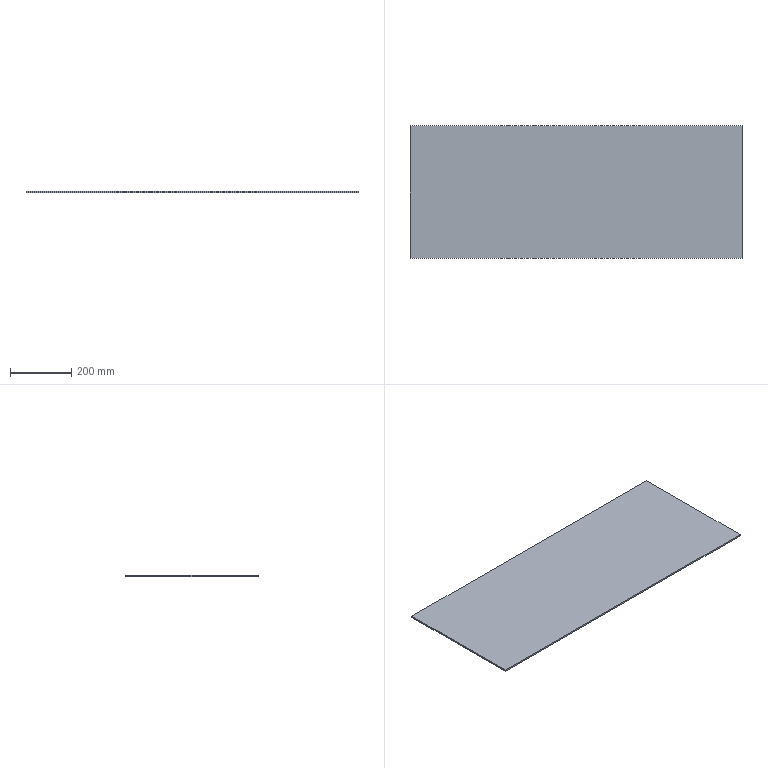Part | STEP file | Vibration-damping sponge | 1 solid | 6 faces | box 1080 x 430 x 5 mm | volume 2322000 mm3 | plane 6
STEP:
#1=CARTESIAN_POINT('',(0.,0.,0.));
#2=DIRECTION('',(0.,0.,1.));
#3=DIRECTION('',(1.,0.,0.));
#4=AXIS2_PLACEMENT_3D('',#1,#2,#3);
#5=CARTESIAN_POINT('',(-540.,215.,0.));
#6=VERTEX_POINT('',#5);
#7=CARTESIAN_POINT('',(-540.,-215.,0.));
#8=VERTEX_POINT('',#7);
#9=CARTESIAN_POINT('',(-540.,215.,0.));
#10=DIRECTION('',(0.,-1.,0.));
#11=VECTOR('',#10,1.);
#12=LINE('',#9,#11);
#13=CARTESIAN_POINT('',(-540.,215.,5.));
#14=DIRECTION('',(1.,0.,0.));
#15=DIRECTION('',(0.,0.,-1.));
#16=AXIS2_PLACEMENT_3D('',#13,#14,#15);
#17=PLANE('',#16);
#18=CARTESIAN_POINT('',(5.,0.));
#19=DIRECTION('',(0.,-1.));
#20=VECTOR('',#19,1.);
#21=LINE('',#18,#20);
#22=(GEOMETRIC_REPRESENTATION_CONTEXT(2)PARAMETRIC_REPRESENTATION_CONTEXT()REPRESENTATION_CONTEXT('',''));
#23=DEFINITIONAL_REPRESENTATION('',(#21),#22);
#24=PCURVE('',#17,#23);
#25=CARTESIAN_POINT('',(-540.,-215.,0.));
#26=DIRECTION('',(0.,0.,1.));
#27=DIRECTION('',(1.,0.,0.));
#28=AXIS2_PLACEMENT_3D('',#25,#26,#27);
#29=PLANE('',#28);
#30=CARTESIAN_POINT('',(0.,430.));
#31=DIRECTION('',(0.,-1.));
#32=VECTOR('',#31,1.);
#33=LINE('',#30,#32);
#34=(GEOMETRIC_REPRESENTATION_CONTEXT(2)PARAMETRIC_REPRESENTATION_CONTEXT()REPRESENTATION_CONTEXT('',''));
#35=DEFINITIONAL_REPRESENTATION('',(#33),#34);
#36=PCURVE('',#29,#35);
#37=SURFACE_CURVE('',#12,(#24,#36),.PCURVE_S1.);
#38=EDGE_CURVE('',#6,#8,#37,.T.);
#39=ORIENTED_EDGE('',*,*,#38,.T.);
#40=CARTESIAN_POINT('',(-540.,-215.,5.));
#41=VERTEX_POINT('',#40);
#42=CARTESIAN_POINT('',(-540.,-215.,5.));
#43=DIRECTION('',(0.,0.,-1.));
#44=VECTOR('',#43,1.);
#45=LINE('',#42,#44);
#46=CARTESIAN_POINT('',(0.,-430.));
#47=DIRECTION('',(1.,0.));
#48=VECTOR('',#47,1.);
#49=LINE('',#46,#48);
#50=(GEOMETRIC_REPRESENTATION_CONTEXT(2)PARAMETRIC_REPRESENTATION_CONTEXT()REPRESENTATION_CONTEXT('',''));
#51=DEFINITIONAL_REPRESENTATION('',(#49),#50);
#52=PCURVE('',#17,#51);
#53=CARTESIAN_POINT('',(-540.,-215.,5.));
#54=DIRECTION('',(0.,1.,0.));
#55=DIRECTION('',(0.,0.,1.));
#56=AXIS2_PLACEMENT_3D('',#53,#54,#55);
#57=PLANE('',#56);
#58=CARTESIAN_POINT('',(0.,0.));
#59=DIRECTION('',(-1.,0.));
#60=VECTOR('',#59,1.);
#61=LINE('',#58,#60);
#62=(GEOMETRIC_REPRESENTATION_CONTEXT(2)PARAMETRIC_REPRESENTATION_CONTEXT()REPRESENTATION_CONTEXT('',''));
#63=DEFINITIONAL_REPRESENTATION('',(#61),#62);
#64=PCURVE('',#57,#63);
#65=SURFACE_CURVE('',#45,(#52,#64),.PCURVE_S1.);
#66=EDGE_CURVE('',#41,#8,#65,.T.);
#67=ORIENTED_EDGE('',*,*,#66,.F.);
#68=CARTESIAN_POINT('',(-540.,215.,5.));
#69=VERTEX_POINT('',#68);
#70=CARTESIAN_POINT('',(-540.,215.,5.));
#71=DIRECTION('',(0.,-1.,0.));
#72=VECTOR('',#71,1.);
#73=LINE('',#70,#72);
#74=CARTESIAN_POINT('',(0.,0.));
#75=DIRECTION('',(0.,-1.));
#76=VECTOR('',#75,1.);
#77=LINE('',#74,#76);
#78=(GEOMETRIC_REPRESENTATION_CONTEXT(2)PARAMETRIC_REPRESENTATION_CONTEXT()REPRESENTATION_CONTEXT('',''));
#79=DEFINITIONAL_REPRESENTATION('',(#77),#78);
#80=PCURVE('',#17,#79);
#81=CARTESIAN_POINT('',(-540.,-215.,5.));
#82=DIRECTION('',(0.,0.,1.));
#83=DIRECTION('',(1.,0.,0.));
#84=AXIS2_PLACEMENT_3D('',#81,#82,#83);
#85=PLANE('',#84);
#86=CARTESIAN_POINT('',(0.,430.));
#87=DIRECTION('',(0.,-1.));
#88=VECTOR('',#87,1.);
#89=LINE('',#86,#88);
#90=(GEOMETRIC_REPRESENTATION_CONTEXT(2)PARAMETRIC_REPRESENTATION_CONTEXT()REPRESENTATION_CONTEXT('',''));
#91=DEFINITIONAL_REPRESENTATION('',(#89),#90);
#92=PCURVE('',#85,#91);
#93=SURFACE_CURVE('',#73,(#80,#92),.PCURVE_S1.);
#94=EDGE_CURVE('',#69,#41,#93,.T.);
#95=ORIENTED_EDGE('',*,*,#94,.F.);
#96=CARTESIAN_POINT('',(-540.,215.,5.));
#97=DIRECTION('',(0.,0.,-1.));
#98=VECTOR('',#97,1.);
#99=LINE('',#96,#98);
#100=CARTESIAN_POINT('',(0.,0.));
#101=DIRECTION('',(1.,0.));
#102=VECTOR('',#101,1.);
#103=LINE('',#100,#102);
#104=(GEOMETRIC_REPRESENTATION_CONTEXT(2)PARAMETRIC_REPRESENTATION_CONTEXT()REPRESENTATION_CONTEXT('',''));
#105=DEFINITIONAL_REPRESENTATION('',(#103),#104);
#106=PCURVE('',#17,#105);
#107=CARTESIAN_POINT('',(-540.,215.,5.));
#108=DIRECTION('',(0.,-1.,0.));
#109=DIRECTION('',(0.,0.,-1.));
#110=AXIS2_PLACEMENT_3D('',#107,#108,#109);
#111=PLANE('',#110);
#112=CARTESIAN_POINT('',(0.,0.));
#113=DIRECTION('',(1.,0.));
#114=VECTOR('',#113,1.);
#115=LINE('',#112,#114);
#116=(GEOMETRIC_REPRESENTATION_CONTEXT(2)PARAMETRIC_REPRESENTATION_CONTEXT()REPRESENTATION_CONTEXT('',''));
#117=DEFINITIONAL_REPRESENTATION('',(#115),#116);
#118=PCURVE('',#111,#117);
#119=SURFACE_CURVE('',#99,(#106,#118),.PCURVE_S1.);
#120=EDGE_CURVE('',#69,#6,#119,.T.);
#121=ORIENTED_EDGE('',*,*,#120,.T.);
#122=EDGE_LOOP('',(#39,#67,#95,#121));
#123=FACE_BOUND('',#122,.T.);
#124=ADVANCED_FACE('',(#123),#17,.F.);
#125=CARTESIAN_POINT('',(540.,-215.,0.));
#126=VERTEX_POINT('',#125);
#127=CARTESIAN_POINT('',(-540.,-215.,0.));
#128=DIRECTION('',(1.,0.,0.));
#129=VECTOR('',#128,1.);
#130=LINE('',#127,#129);
#131=CARTESIAN_POINT('',(-5.,0.));
#132=DIRECTION('',(0.,1.));
#133=VECTOR('',#132,1.);
#134=LINE('',#131,#133);
#135=(GEOMETRIC_REPRESENTATION_CONTEXT(2)PARAMETRIC_REPRESENTATION_CONTEXT()REPRESENTATION_CONTEXT('',''));
#136=DEFINITIONAL_REPRESENTATION('',(#134),#135);
#137=PCURVE('',#57,#136);
#138=CARTESIAN_POINT('',(0.,0.));
#139=DIRECTION('',(1.,0.));
#140=VECTOR('',#139,1.);
#141=LINE('',#138,#140);
#142=(GEOMETRIC_REPRESENTATION_CONTEXT(2)PARAMETRIC_REPRESENTATION_CONTEXT()REPRESENTATION_CONTEXT('',''));
#143=DEFINITIONAL_REPRESENTATION('',(#141),#142);
#144=PCURVE('',#29,#143);
#145=SURFACE_CURVE('',#130,(#137,#144),.PCURVE_S1.);
#146=EDGE_CURVE('',#8,#126,#145,.T.);
#147=ORIENTED_EDGE('',*,*,#146,.T.);
#148=CARTESIAN_POINT('',(540.,-215.,5.));
#149=VERTEX_POINT('',#148);
#150=CARTESIAN_POINT('',(540.,-215.,5.));
#151=DIRECTION('',(0.,0.,-1.));
#152=VECTOR('',#151,1.);
#153=LINE('',#150,#152);
#154=CARTESIAN_POINT('',(0.,1080.));
#155=DIRECTION('',(-1.,0.));
#156=VECTOR('',#155,1.);
#157=LINE('',#154,#156);
#158=(GEOMETRIC_REPRESENTATION_CONTEXT(2)PARAMETRIC_REPRESENTATION_CONTEXT()REPRESENTATION_CONTEXT('',''));
#159=DEFINITIONAL_REPRESENTATION('',(#157),#158);
#160=PCURVE('',#57,#159);
#161=CARTESIAN_POINT('',(540.,215.,5.));
#162=DIRECTION('',(-1.,0.,0.));
#163=DIRECTION('',(0.,0.,1.));
#164=AXIS2_PLACEMENT_3D('',#161,#162,#163);
#165=PLANE('',#164);
#166=CARTESIAN_POINT('',(0.,-430.));
#167=DIRECTION('',(-1.,0.));
#168=VECTOR('',#167,1.);
#169=LINE('',#166,#168);
#170=(GEOMETRIC_REPRESENTATION_CONTEXT(2)PARAMETRIC_REPRESENTATION_CONTEXT()REPRESENTATION_CONTEXT('',''));
#171=DEFINITIONAL_REPRESENTATION('',(#169),#170);
#172=PCURVE('',#165,#171);
#173=SURFACE_CURVE('',#153,(#160,#172),.PCURVE_S1.);
#174=EDGE_CURVE('',#149,#126,#173,.T.);
#175=ORIENTED_EDGE('',*,*,#174,.F.);
#176=CARTESIAN_POINT('',(-540.,-215.,5.));
#177=DIRECTION('',(1.,0.,0.));
#178=VECTOR('',#177,1.);
#179=LINE('',#176,#178);
#180=CARTESIAN_POINT('',(0.,0.));
#181=DIRECTION('',(0.,1.));
#182=VECTOR('',#181,1.);
#183=LINE('',#180,#182);
#184=(GEOMETRIC_REPRESENTATION_CONTEXT(2)PARAMETRIC_REPRESENTATION_CONTEXT()REPRESENTATION_CONTEXT('',''));
#185=DEFINITIONAL_REPRESENTATION('',(#183),#184);
#186=PCURVE('',#57,#185);
#187=CARTESIAN_POINT('',(0.,0.));
#188=DIRECTION('',(1.,0.));
#189=VECTOR('',#188,1.);
#190=LINE('',#187,#189);
#191=(GEOMETRIC_REPRESENTATION_CONTEXT(2)PARAMETRIC_REPRESENTATION_CONTEXT()REPRESENTATION_CONTEXT('',''));
#192=DEFINITIONAL_REPRESENTATION('',(#190),#191);
#193=PCURVE('',#85,#192);
#194=SURFACE_CURVE('',#179,(#186,#193),.PCURVE_S1.);
#195=EDGE_CURVE('',#41,#149,#194,.T.);
#196=ORIENTED_EDGE('',*,*,#195,.F.);
#197=ORIENTED_EDGE('',*,*,#66,.T.);
#198=EDGE_LOOP('',(#147,#175,#196,#197));
#199=FACE_BOUND('',#198,.T.);
#200=ADVANCED_FACE('',(#199),#57,.F.);
#201=CARTESIAN_POINT('',(540.,215.,0.));
#202=VERTEX_POINT('',#201);
#203=CARTESIAN_POINT('',(540.,215.,0.));
#204=DIRECTION('',(0.,1.,0.));
#205=VECTOR('',#204,1.);
#206=LINE('',#203,#205);
#207=CARTESIAN_POINT('',(-5.,0.));
#208=DIRECTION('',(0.,1.));
#209=VECTOR('',#208,1.);
#210=LINE('',#207,#209);
#211=(GEOMETRIC_REPRESENTATION_CONTEXT(2)PARAMETRIC_REPRESENTATION_CONTEXT()REPRESENTATION_CONTEXT('',''));
#212=DEFINITIONAL_REPRESENTATION('',(#210),#211);
#213=PCURVE('',#165,#212);
#214=CARTESIAN_POINT('',(1080.,430.));
#215=DIRECTION('',(0.,1.));
#216=VECTOR('',#215,1.);
#217=LINE('',#214,#216);
#218=(GEOMETRIC_REPRESENTATION_CONTEXT(2)PARAMETRIC_REPRESENTATION_CONTEXT()REPRESENTATION_CONTEXT('',''));
#219=DEFINITIONAL_REPRESENTATION('',(#217),#218);
#220=PCURVE('',#29,#219);
#221=SURFACE_CURVE('',#206,(#213,#220),.PCURVE_S1.);
#222=EDGE_CURVE('',#126,#202,#221,.T.);
#223=ORIENTED_EDGE('',*,*,#222,.T.);
#224=CARTESIAN_POINT('',(540.,215.,5.));
#225=VERTEX_POINT('',#224);
#226=CARTESIAN_POINT('',(540.,215.,5.));
#227=DIRECTION('',(0.,0.,-1.));
#228=VECTOR('',#227,1.);
#229=LINE('',#226,#228);
#230=CARTESIAN_POINT('',(0.,0.));
#231=DIRECTION('',(-1.,0.));
#232=VECTOR('',#231,1.);
#233=LINE('',#230,#232);
#234=(GEOMETRIC_REPRESENTATION_CONTEXT(2)PARAMETRIC_REPRESENTATION_CONTEXT()REPRESENTATION_CONTEXT('',''));
#235=DEFINITIONAL_REPRESENTATION('',(#233),#234);
#236=PCURVE('',#165,#235);
#237=CARTESIAN_POINT('',(0.,1080.));
#238=DIRECTION('',(1.,0.));
#239=VECTOR('',#238,1.);
#240=LINE('',#237,#239);
#241=(GEOMETRIC_REPRESENTATION_CONTEXT(2)PARAMETRIC_REPRESENTATION_CONTEXT()REPRESENTATION_CONTEXT('',''));
#242=DEFINITIONAL_REPRESENTATION('',(#240),#241);
#243=PCURVE('',#111,#242);
#244=SURFACE_CURVE('',#229,(#236,#243),.PCURVE_S1.);
#245=EDGE_CURVE('',#225,#202,#244,.T.);
#246=ORIENTED_EDGE('',*,*,#245,.F.);
#247=CARTESIAN_POINT('',(540.,215.,5.));
#248=DIRECTION('',(0.,1.,0.));
#249=VECTOR('',#248,1.);
#250=LINE('',#247,#249);
#251=CARTESIAN_POINT('',(0.,0.));
#252=DIRECTION('',(0.,1.));
#253=VECTOR('',#252,1.);
#254=LINE('',#251,#253);
#255=(GEOMETRIC_REPRESENTATION_CONTEXT(2)PARAMETRIC_REPRESENTATION_CONTEXT()REPRESENTATION_CONTEXT('',''));
#256=DEFINITIONAL_REPRESENTATION('',(#254),#255);
#257=PCURVE('',#165,#256);
#258=CARTESIAN_POINT('',(1080.,430.));
#259=DIRECTION('',(0.,1.));
#260=VECTOR('',#259,1.);
#261=LINE('',#258,#260);
#262=(GEOMETRIC_REPRESENTATION_CONTEXT(2)PARAMETRIC_REPRESENTATION_CONTEXT()REPRESENTATION_CONTEXT('',''));
#263=DEFINITIONAL_REPRESENTATION('',(#261),#262);
#264=PCURVE('',#85,#263);
#265=SURFACE_CURVE('',#250,(#257,#264),.PCURVE_S1.);
#266=EDGE_CURVE('',#149,#225,#265,.T.);
#267=ORIENTED_EDGE('',*,*,#266,.F.);
#268=ORIENTED_EDGE('',*,*,#174,.T.);
#269=EDGE_LOOP('',(#223,#246,#267,#268));
#270=FACE_BOUND('',#269,.T.);
#271=ADVANCED_FACE('',(#270),#165,.F.);
#272=CARTESIAN_POINT('',(-540.,215.,0.));
#273=DIRECTION('',(-1.,0.,0.));
#274=VECTOR('',#273,1.);
#275=LINE('',#272,#274);
#276=CARTESIAN_POINT('',(5.,0.));
#277=DIRECTION('',(0.,-1.));
#278=VECTOR('',#277,1.);
#279=LINE('',#276,#278);
#280=(GEOMETRIC_REPRESENTATION_CONTEXT(2)PARAMETRIC_REPRESENTATION_CONTEXT()REPRESENTATION_CONTEXT('',''));
#281=DEFINITIONAL_REPRESENTATION('',(#279),#280);
#282=PCURVE('',#111,#281);
#283=CARTESIAN_POINT('',(0.,430.));
#284=DIRECTION('',(-1.,0.));
#285=VECTOR('',#284,1.);
#286=LINE('',#283,#285);
#287=(GEOMETRIC_REPRESENTATION_CONTEXT(2)PARAMETRIC_REPRESENTATION_CONTEXT()REPRESENTATION_CONTEXT('',''));
#288=DEFINITIONAL_REPRESENTATION('',(#286),#287);
#289=PCURVE('',#29,#288);
#290=SURFACE_CURVE('',#275,(#282,#289),.PCURVE_S1.);
#291=EDGE_CURVE('',#202,#6,#290,.T.);
#292=ORIENTED_EDGE('',*,*,#291,.T.);
#293=ORIENTED_EDGE('',*,*,#120,.F.);
#294=CARTESIAN_POINT('',(-540.,215.,5.));
#295=DIRECTION('',(-1.,0.,0.));
#296=VECTOR('',#295,1.);
#297=LINE('',#294,#296);
#298=CARTESIAN_POINT('',(0.,0.));
#299=DIRECTION('',(0.,-1.));
#300=VECTOR('',#299,1.);
#301=LINE('',#298,#300);
#302=(GEOMETRIC_REPRESENTATION_CONTEXT(2)PARAMETRIC_REPRESENTATION_CONTEXT()REPRESENTATION_CONTEXT('',''));
#303=DEFINITIONAL_REPRESENTATION('',(#301),#302);
#304=PCURVE('',#111,#303);
#305=CARTESIAN_POINT('',(0.,430.));
#306=DIRECTION('',(-1.,0.));
#307=VECTOR('',#306,1.);
#308=LINE('',#305,#307);
#309=(GEOMETRIC_REPRESENTATION_CONTEXT(2)PARAMETRIC_REPRESENTATION_CONTEXT()REPRESENTATION_CONTEXT('',''));
#310=DEFINITIONAL_REPRESENTATION('',(#308),#309);
#311=PCURVE('',#85,#310);
#312=SURFACE_CURVE('',#297,(#304,#311),.PCURVE_S1.);
#313=EDGE_CURVE('',#225,#69,#312,.T.);
#314=ORIENTED_EDGE('',*,*,#313,.F.);
#315=ORIENTED_EDGE('',*,*,#245,.T.);
#316=EDGE_LOOP('',(#292,#293,#314,#315));
#317=FACE_BOUND('',#316,.T.);
#318=ADVANCED_FACE('',(#317),#111,.F.);
#319=ORIENTED_EDGE('',*,*,#94,.T.);
#320=ORIENTED_EDGE('',*,*,#195,.T.);
#321=ORIENTED_EDGE('',*,*,#266,.T.);
#322=ORIENTED_EDGE('',*,*,#313,.T.);
#323=EDGE_LOOP('',(#319,#320,#321,#322));
#324=FACE_BOUND('',#323,.T.);
#325=ADVANCED_FACE('',(#324),#85,.T.);
#326=ORIENTED_EDGE('',*,*,#38,.F.);
#327=ORIENTED_EDGE('',*,*,#291,.F.);
#328=ORIENTED_EDGE('',*,*,#222,.F.);
#329=ORIENTED_EDGE('',*,*,#146,.F.);
#330=EDGE_LOOP('',(#326,#327,#328,#329));
#331=FACE_BOUND('',#330,.T.);
#332=ADVANCED_FACE('',(#331),#29,.F.);
#333=CLOSED_SHELL('',(#124,#200,#271,#318,#325,#332));
#334=MANIFOLD_SOLID_BREP('',#333);
#335=(LENGTH_UNIT()NAMED_UNIT(*)SI_UNIT(.MILLI.,.METRE.));
#336=UNCERTAINTY_MEASURE_WITH_UNIT(LENGTH_MEASURE(0.0000001),#335,'','');
#337=(NAMED_UNIT(*)PLANE_ANGLE_UNIT()SI_UNIT($,.RADIAN.));
#338=(NAMED_UNIT(*)SI_UNIT($,.STERADIAN.)SOLID_ANGLE_UNIT());
#339=(GEOMETRIC_REPRESENTATION_CONTEXT(3)GLOBAL_UNCERTAINTY_ASSIGNED_CONTEXT((#336))GLOBAL_UNIT_ASSIGNED_CONTEXT((#335,#337,#338))REPRESENTATION_CONTEXT('',''));
#340=ADVANCED_BREP_SHAPE_REPRESENTATION('',(#4,#334),#339);